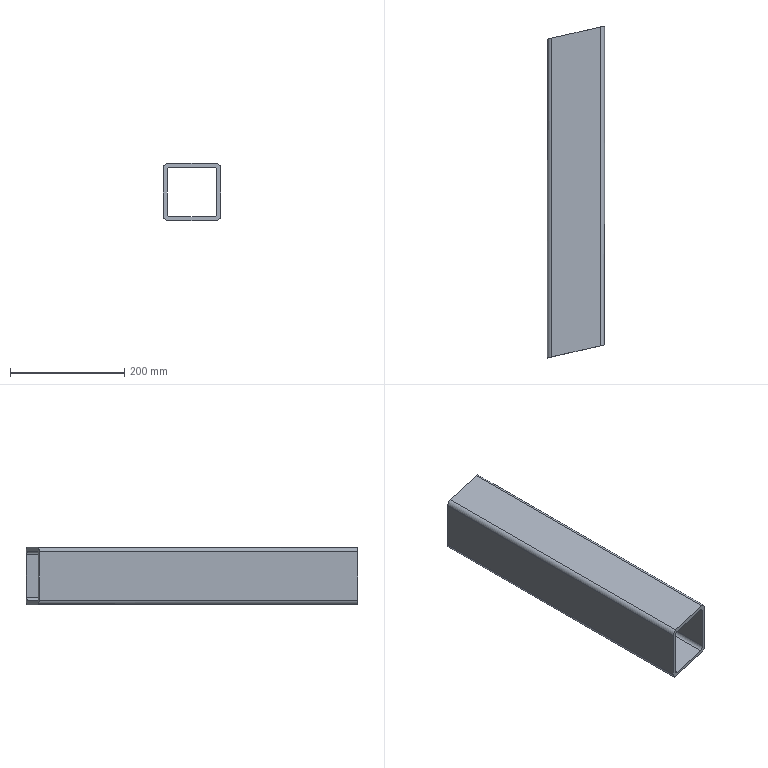Part | SolidWorks | features Extrusion 1, ICE 1 | 1 solid | 18 faces | box 100 x 582 x 100 mm | volume 1309220 mm3 | plane 10 | cylinder 8 | commonest cylinder face diameters 12.6 x4 15.75 x4
STEP:
#1=CARTESIAN_POINT('',(100.,291.,-90.6));
#2=VERTEX_POINT('',#1);
#3=CARTESIAN_POINT('',(100.,-268.,-90.6));
#4=VERTEX_POINT('',#3);
#5=CARTESIAN_POINT('',(100.,291.,-90.6));
#6=DIRECTION('',(0.,-1.,0.));
#7=VECTOR('',#6,1000.);
#8=LINE('',#5,#7);
#9=EDGE_CURVE('',#2,#4,#8,.T.);
#10=ORIENTED_EDGE('',*,*,#9,.T.);
#11=CARTESIAN_POINT('',(92.125,-269.811,-98.475));
#12=VERTEX_POINT('',#11);
#13=CARTESIAN_POINT('',(92.125,-269.811,-98.475));
#14=CARTESIAN_POINT('',(96.738,-268.75,-98.475));
#15=CARTESIAN_POINT('',(100.,-268.,-95.213));
#16=CARTESIAN_POINT('',(100.,-268.,-90.6));
#17=(BOUNDED_CURVE()B_SPLINE_CURVE(3,(#13,#14,#15,#16),.UNSPECIFIED.,.F.,.T.)B_SPLINE_CURVE_WITH_KNOTS((4,4),(1.571,3.142),.UNSPECIFIED.)CURVE()GEOMETRIC_REPRESENTATION_ITEM()RATIONAL_B_SPLINE_CURVE((1.,0.8047,0.8047,1.))REPRESENTATION_ITEM(''));
#18=EDGE_CURVE('',#12,#4,#17,.T.);
#19=ORIENTED_EDGE('',*,*,#18,.F.);
#20=CARTESIAN_POINT('',(92.125,289.189,-98.475));
#21=VERTEX_POINT('',#20);
#22=CARTESIAN_POINT('',(92.125,291.,-98.475));
#23=DIRECTION('',(0.,-1.,0.));
#24=VECTOR('',#23,1000.);
#25=LINE('',#22,#24);
#26=EDGE_CURVE('',#21,#12,#25,.T.);
#27=ORIENTED_EDGE('',*,*,#26,.F.);
#28=CARTESIAN_POINT('',(100.,291.,-90.6));
#29=CARTESIAN_POINT('',(100.,291.,-95.213));
#30=CARTESIAN_POINT('',(96.738,290.25,-98.475));
#31=CARTESIAN_POINT('',(92.125,289.189,-98.475));
#32=(BOUNDED_CURVE()B_SPLINE_CURVE(3,(#28,#29,#30,#31),.UNSPECIFIED.,.F.,.T.)B_SPLINE_CURVE_WITH_KNOTS((4,4),(3.142,4.712),.UNSPECIFIED.)CURVE()GEOMETRIC_REPRESENTATION_ITEM()RATIONAL_B_SPLINE_CURVE((1.,0.8047,0.8047,1.))REPRESENTATION_ITEM(''));
#33=EDGE_CURVE('',#2,#21,#32,.T.);
#34=ORIENTED_EDGE('',*,*,#33,.F.);
#35=EDGE_LOOP('',(#10,#19,#27,#34));
#36=FACE_OUTER_BOUND('',#35,.T.);
#37=CARTESIAN_POINT('',(92.125,291.,-90.6));
#38=DIRECTION('',(0.,-1.,0.));
#39=DIRECTION('',(0.,0.,-1.));
#40=AXIS2_PLACEMENT_3D('',#37,#38,#39);
#41=CYLINDRICAL_SURFACE('',#40,7.875);
#42=ADVANCED_FACE('',(#36),#41,.T.);
#43=ORIENTED_EDGE('',*,*,#26,.T.);
#44=CARTESIAN_POINT('',(7.875,-289.189,-98.475));
#45=VERTEX_POINT('',#44);
#46=CARTESIAN_POINT('',(0.,-291.,-98.475));
#47=DIRECTION('',(0.9746,0.2241,0.));
#48=VECTOR('',#47,1000.);
#49=LINE('',#46,#48);
#50=EDGE_CURVE('',#45,#12,#49,.T.);
#51=ORIENTED_EDGE('',*,*,#50,.F.);
#52=CARTESIAN_POINT('',(7.875,269.811,-98.475));
#53=VERTEX_POINT('',#52);
#54=CARTESIAN_POINT('',(7.875,291.,-98.475));
#55=DIRECTION('',(0.,-1.,0.));
#56=VECTOR('',#55,1000.);
#57=LINE('',#54,#56);
#58=EDGE_CURVE('',#53,#45,#57,.T.);
#59=ORIENTED_EDGE('',*,*,#58,.F.);
#60=CARTESIAN_POINT('',(100.,291.,-98.475));
#61=DIRECTION('',(-0.9746,-0.2241,0.));
#62=VECTOR('',#61,1000.);
#63=LINE('',#60,#62);
#64=EDGE_CURVE('',#21,#53,#63,.T.);
#65=ORIENTED_EDGE('',*,*,#64,.F.);
#66=EDGE_LOOP('',(#43,#51,#59,#65));
#67=FACE_OUTER_BOUND('',#66,.T.);
#68=CARTESIAN_POINT('',(92.125,291.,-98.475));
#69=DIRECTION('',(0.,0.,1.));
#70=DIRECTION('',(1.,0.,0.));
#71=AXIS2_PLACEMENT_3D('',#68,#69,#70);
#72=PLANE('',#71);
#73=ADVANCED_FACE('',(#67),#72,.F.);
#74=ORIENTED_EDGE('',*,*,#58,.T.);
#75=CARTESIAN_POINT('',(0.,-291.,-90.6));
#76=VERTEX_POINT('',#75);
#77=CARTESIAN_POINT('',(0.,-291.,-90.6));
#78=CARTESIAN_POINT('',(0.,-291.,-95.213));
#79=CARTESIAN_POINT('',(3.262,-290.25,-98.475));
#80=CARTESIAN_POINT('',(7.875,-289.189,-98.475));
#81=(BOUNDED_CURVE()B_SPLINE_CURVE(3,(#77,#78,#79,#80),.UNSPECIFIED.,.F.,.T.)B_SPLINE_CURVE_WITH_KNOTS((4,4),(0.,1.571),.UNSPECIFIED.)CURVE()GEOMETRIC_REPRESENTATION_ITEM()RATIONAL_B_SPLINE_CURVE((1.,0.8047,0.8047,1.))REPRESENTATION_ITEM(''));
#82=EDGE_CURVE('',#76,#45,#81,.T.);
#83=ORIENTED_EDGE('',*,*,#82,.F.);
#84=CARTESIAN_POINT('',(0.,268.,-90.6));
#85=VERTEX_POINT('',#84);
#86=CARTESIAN_POINT('',(0.,291.,-90.6));
#87=DIRECTION('',(0.,-1.,0.));
#88=VECTOR('',#87,1000.);
#89=LINE('',#86,#88);
#90=EDGE_CURVE('',#85,#76,#89,.T.);
#91=ORIENTED_EDGE('',*,*,#90,.F.);
#92=CARTESIAN_POINT('',(7.875,269.811,-98.475));
#93=CARTESIAN_POINT('',(3.262,268.75,-98.475));
#94=CARTESIAN_POINT('',(0.,268.,-95.213));
#95=CARTESIAN_POINT('',(0.,268.,-90.6));
#96=(BOUNDED_CURVE()B_SPLINE_CURVE(3,(#92,#93,#94,#95),.UNSPECIFIED.,.F.,.F.)B_SPLINE_CURVE_WITH_KNOTS((4,4),(4.712,6.283),.UNSPECIFIED.)CURVE()GEOMETRIC_REPRESENTATION_ITEM()RATIONAL_B_SPLINE_CURVE((1.,0.8047,0.8047,1.))REPRESENTATION_ITEM(''));
#97=EDGE_CURVE('',#53,#85,#96,.T.);
#98=ORIENTED_EDGE('',*,*,#97,.F.);
#99=EDGE_LOOP('',(#74,#83,#91,#98));
#100=FACE_OUTER_BOUND('',#99,.T.);
#101=CARTESIAN_POINT('',(7.875,291.,-90.6));
#102=DIRECTION('',(0.,-1.,0.));
#103=DIRECTION('',(0.,0.,-1.));
#104=AXIS2_PLACEMENT_3D('',#101,#102,#103);
#105=CYLINDRICAL_SURFACE('',#104,7.875);
#106=ADVANCED_FACE('',(#100),#105,.T.);
#107=CARTESIAN_POINT('',(0.,268.,-6.35));
#108=VERTEX_POINT('',#107);
#109=CARTESIAN_POINT('',(0.,-291.,-6.35));
#110=VERTEX_POINT('',#109);
#111=CARTESIAN_POINT('',(0.,291.,-6.35));
#112=DIRECTION('',(0.,-1.,0.));
#113=VECTOR('',#112,1000.);
#114=LINE('',#111,#113);
#115=EDGE_CURVE('',#108,#110,#114,.T.);
#116=ORIENTED_EDGE('',*,*,#115,.F.);
#117=CARTESIAN_POINT('',(0.,268.,-98.476));
#118=DIRECTION('',(0.,0.,1.));
#119=VECTOR('',#118,1000.);
#120=LINE('',#117,#119);
#121=EDGE_CURVE('',#85,#108,#120,.T.);
#122=ORIENTED_EDGE('',*,*,#121,.F.);
#123=ORIENTED_EDGE('',*,*,#90,.T.);
#124=CARTESIAN_POINT('',(0.,-291.,-6.35));
#125=DIRECTION('',(0.,0.,1.));
#126=VECTOR('',#125,1000.);
#127=LINE('',#124,#126);
#128=EDGE_CURVE('',#76,#110,#127,.T.);
#129=ORIENTED_EDGE('',*,*,#128,.T.);
#130=EDGE_LOOP('',(#116,#122,#123,#129));
#131=FACE_OUTER_BOUND('',#130,.T.);
#132=CARTESIAN_POINT('',(0.,291.,-6.35));
#133=DIRECTION('',(1.,0.,0.));
#134=DIRECTION('',(0.,0.,-1.));
#135=AXIS2_PLACEMENT_3D('',#132,#133,#134);
#136=PLANE('',#135);
#137=ADVANCED_FACE('',(#131),#136,.F.);
#138=ORIENTED_EDGE('',*,*,#115,.T.);
#139=CARTESIAN_POINT('',(7.875,-289.189,1.525));
#140=VERTEX_POINT('',#139);
#141=CARTESIAN_POINT('',(7.875,-289.189,1.525));
#142=CARTESIAN_POINT('',(3.262,-290.25,1.525));
#143=CARTESIAN_POINT('',(0.,-291.,-1.737));
#144=CARTESIAN_POINT('',(0.,-291.,-6.35));
#145=(BOUNDED_CURVE()B_SPLINE_CURVE(3,(#141,#142,#143,#144),.UNSPECIFIED.,.F.,.T.)B_SPLINE_CURVE_WITH_KNOTS((4,4),(4.712,6.283),.UNSPECIFIED.)CURVE()GEOMETRIC_REPRESENTATION_ITEM()RATIONAL_B_SPLINE_CURVE((1.,0.8047,0.8047,1.))REPRESENTATION_ITEM(''));
#146=EDGE_CURVE('',#140,#110,#145,.T.);
#147=ORIENTED_EDGE('',*,*,#146,.F.);
#148=CARTESIAN_POINT('',(7.875,269.811,1.525));
#149=VERTEX_POINT('',#148);
#150=CARTESIAN_POINT('',(7.875,291.,1.525));
#151=DIRECTION('',(0.,-1.,0.));
#152=VECTOR('',#151,1000.);
#153=LINE('',#150,#152);
#154=EDGE_CURVE('',#149,#140,#153,.T.);
#155=ORIENTED_EDGE('',*,*,#154,.F.);
#156=CARTESIAN_POINT('',(0.,268.,-6.35));
#157=CARTESIAN_POINT('',(0.,268.,-1.737));
#158=CARTESIAN_POINT('',(3.262,268.75,1.525));
#159=CARTESIAN_POINT('',(7.875,269.811,1.525));
#160=(BOUNDED_CURVE()B_SPLINE_CURVE(3,(#156,#157,#158,#159),.UNSPECIFIED.,.F.,.T.)B_SPLINE_CURVE_WITH_KNOTS((4,4),(0.,1.571),.UNSPECIFIED.)CURVE()GEOMETRIC_REPRESENTATION_ITEM()RATIONAL_B_SPLINE_CURVE((1.,0.8047,0.8047,1.))REPRESENTATION_ITEM(''));
#161=EDGE_CURVE('',#108,#149,#160,.T.);
#162=ORIENTED_EDGE('',*,*,#161,.F.);
#163=EDGE_LOOP('',(#138,#147,#155,#162));
#164=FACE_OUTER_BOUND('',#163,.T.);
#165=CARTESIAN_POINT('',(7.875,291.,-6.35));
#166=DIRECTION('',(0.,-1.,0.));
#167=DIRECTION('',(0.,0.,-1.));
#168=AXIS2_PLACEMENT_3D('',#165,#166,#167);
#169=CYLINDRICAL_SURFACE('',#168,7.875);
#170=ADVANCED_FACE('',(#164),#169,.T.);
#171=ORIENTED_EDGE('',*,*,#154,.T.);
#172=CARTESIAN_POINT('',(92.125,-269.811,1.525));
#173=VERTEX_POINT('',#172);
#174=CARTESIAN_POINT('',(0.,-291.,1.525));
#175=DIRECTION('',(-0.9746,-0.2241,0.));
#176=VECTOR('',#175,1000.);
#177=LINE('',#174,#176);
#178=EDGE_CURVE('',#173,#140,#177,.T.);
#179=ORIENTED_EDGE('',*,*,#178,.F.);
#180=CARTESIAN_POINT('',(92.125,289.189,1.525));
#181=VERTEX_POINT('',#180);
#182=CARTESIAN_POINT('',(92.125,291.,1.525));
#183=DIRECTION('',(0.,-1.,0.));
#184=VECTOR('',#183,1000.);
#185=LINE('',#182,#184);
#186=EDGE_CURVE('',#181,#173,#185,.T.);
#187=ORIENTED_EDGE('',*,*,#186,.F.);
#188=CARTESIAN_POINT('',(100.,291.,1.525));
#189=DIRECTION('',(0.9746,0.2241,0.));
#190=VECTOR('',#189,1000.);
#191=LINE('',#188,#190);
#192=EDGE_CURVE('',#149,#181,#191,.T.);
#193=ORIENTED_EDGE('',*,*,#192,.F.);
#194=EDGE_LOOP('',(#171,#179,#187,#193));
#195=FACE_OUTER_BOUND('',#194,.T.);
#196=CARTESIAN_POINT('',(7.875,291.,1.525));
#197=DIRECTION('',(0.,0.,-1.));
#198=DIRECTION('',(-1.,0.,0.));
#199=AXIS2_PLACEMENT_3D('',#196,#197,#198);
#200=PLANE('',#199);
#201=ADVANCED_FACE('',(#195),#200,.F.);
#202=ORIENTED_EDGE('',*,*,#186,.T.);
#203=CARTESIAN_POINT('',(100.,-268.,-6.35));
#204=VERTEX_POINT('',#203);
#205=CARTESIAN_POINT('',(100.,-268.,-6.35));
#206=CARTESIAN_POINT('',(100.,-268.,-1.737));
#207=CARTESIAN_POINT('',(96.738,-268.75,1.525));
#208=CARTESIAN_POINT('',(92.125,-269.811,1.525));
#209=(BOUNDED_CURVE()B_SPLINE_CURVE(3,(#205,#206,#207,#208),.UNSPECIFIED.,.F.,.T.)B_SPLINE_CURVE_WITH_KNOTS((4,4),(3.142,4.712),.UNSPECIFIED.)CURVE()GEOMETRIC_REPRESENTATION_ITEM()RATIONAL_B_SPLINE_CURVE((1.,0.8047,0.8047,1.))REPRESENTATION_ITEM(''));
#210=EDGE_CURVE('',#204,#173,#209,.T.);
#211=ORIENTED_EDGE('',*,*,#210,.F.);
#212=CARTESIAN_POINT('',(100.,291.,-6.35));
#213=VERTEX_POINT('',#212);
#214=CARTESIAN_POINT('',(100.,291.,-6.35));
#215=DIRECTION('',(0.,-1.,0.));
#216=VECTOR('',#215,1000.);
#217=LINE('',#214,#216);
#218=EDGE_CURVE('',#213,#204,#217,.T.);
#219=ORIENTED_EDGE('',*,*,#218,.F.);
#220=CARTESIAN_POINT('',(92.125,289.189,1.525));
#221=CARTESIAN_POINT('',(96.738,290.25,1.525));
#222=CARTESIAN_POINT('',(100.,291.,-1.737));
#223=CARTESIAN_POINT('',(100.,291.,-6.35));
#224=(BOUNDED_CURVE()B_SPLINE_CURVE(3,(#220,#221,#222,#223),.UNSPECIFIED.,.F.,.T.)B_SPLINE_CURVE_WITH_KNOTS((4,4),(1.571,3.142),.UNSPECIFIED.)CURVE()GEOMETRIC_REPRESENTATION_ITEM()RATIONAL_B_SPLINE_CURVE((1.,0.8047,0.8047,1.))REPRESENTATION_ITEM(''));
#225=EDGE_CURVE('',#181,#213,#224,.T.);
#226=ORIENTED_EDGE('',*,*,#225,.F.);
#227=EDGE_LOOP('',(#202,#211,#219,#226));
#228=FACE_OUTER_BOUND('',#227,.T.);
#229=CARTESIAN_POINT('',(92.125,291.,-6.35));
#230=DIRECTION('',(0.,-1.,0.));
#231=DIRECTION('',(0.,0.,-1.));
#232=AXIS2_PLACEMENT_3D('',#229,#230,#231);
#233=CYLINDRICAL_SURFACE('',#232,7.875);
#234=ADVANCED_FACE('',(#228),#233,.T.);
#235=ORIENTED_EDGE('',*,*,#218,.T.);
#236=CARTESIAN_POINT('',(100.,-268.,-98.476));
#237=DIRECTION('',(0.,0.,1.));
#238=VECTOR('',#237,1000.);
#239=LINE('',#236,#238);
#240=EDGE_CURVE('',#4,#204,#239,.T.);
#241=ORIENTED_EDGE('',*,*,#240,.F.);
#242=ORIENTED_EDGE('',*,*,#9,.F.);
#243=CARTESIAN_POINT('',(100.,291.,-90.6));
#244=DIRECTION('',(0.,0.,-1.));
#245=VECTOR('',#244,1000.);
#246=LINE('',#243,#245);
#247=EDGE_CURVE('',#213,#2,#246,.T.);
#248=ORIENTED_EDGE('',*,*,#247,.F.);
#249=EDGE_LOOP('',(#235,#241,#242,#248));
#250=FACE_OUTER_BOUND('',#249,.T.);
#251=CARTESIAN_POINT('',(100.,291.,-90.6));
#252=DIRECTION('',(-1.,0.,0.));
#253=DIRECTION('',(0.,0.,1.));
#254=AXIS2_PLACEMENT_3D('',#251,#252,#253);
#255=PLANE('',#254);
#256=ADVANCED_FACE('',(#250),#255,.F.);
#257=CARTESIAN_POINT('',(6.3,-289.551,-85.875));
#258=VERTEX_POINT('',#257);
#259=CARTESIAN_POINT('',(12.6,-288.102,-92.175));
#260=VERTEX_POINT('',#259);
#261=CARTESIAN_POINT('',(6.3,-289.551,-85.875));
#262=CARTESIAN_POINT('',(6.3,-289.551,-89.565));
#263=CARTESIAN_POINT('',(8.91,-288.951,-92.175));
#264=CARTESIAN_POINT('',(12.6,-288.102,-92.175));
#265=(BOUNDED_CURVE()B_SPLINE_CURVE(3,(#261,#262,#263,#264),.UNSPECIFIED.,.F.,.T.)B_SPLINE_CURVE_WITH_KNOTS((4,4),(0.,1.571),.UNSPECIFIED.)CURVE()GEOMETRIC_REPRESENTATION_ITEM()RATIONAL_B_SPLINE_CURVE((1.,0.8047,0.8047,1.))REPRESENTATION_ITEM(''));
#266=EDGE_CURVE('',#258,#260,#265,.T.);
#267=ORIENTED_EDGE('',*,*,#266,.T.);
#268=CARTESIAN_POINT('',(12.6,270.898,-92.175));
#269=VERTEX_POINT('',#268);
#270=CARTESIAN_POINT('',(12.6,291.,-92.175));
#271=DIRECTION('',(0.,-1.,0.));
#272=VECTOR('',#271,1000.);
#273=LINE('',#270,#272);
#274=EDGE_CURVE('',#269,#260,#273,.T.);
#275=ORIENTED_EDGE('',*,*,#274,.F.);
#276=CARTESIAN_POINT('',(6.3,269.449,-85.875));
#277=VERTEX_POINT('',#276);
#278=CARTESIAN_POINT('',(12.6,270.898,-92.175));
#279=CARTESIAN_POINT('',(8.91,270.049,-92.175));
#280=CARTESIAN_POINT('',(6.3,269.449,-89.565));
#281=CARTESIAN_POINT('',(6.3,269.449,-85.875));
#282=(BOUNDED_CURVE()B_SPLINE_CURVE(3,(#278,#279,#280,#281),.UNSPECIFIED.,.F.,.T.)B_SPLINE_CURVE_WITH_KNOTS((4,4),(4.712,6.283),.UNSPECIFIED.)CURVE()GEOMETRIC_REPRESENTATION_ITEM()RATIONAL_B_SPLINE_CURVE((1.,0.8047,0.8047,1.))REPRESENTATION_ITEM(''));
#283=EDGE_CURVE('',#269,#277,#282,.T.);
#284=ORIENTED_EDGE('',*,*,#283,.T.);
#285=CARTESIAN_POINT('',(6.3,291.,-85.875));
#286=DIRECTION('',(0.,-1.,0.));
#287=VECTOR('',#286,1000.);
#288=LINE('',#285,#287);
#289=EDGE_CURVE('',#277,#258,#288,.T.);
#290=ORIENTED_EDGE('',*,*,#289,.T.);
#291=EDGE_LOOP('',(#267,#275,#284,#290));
#292=FACE_OUTER_BOUND('',#291,.T.);
#293=CARTESIAN_POINT('',(12.6,291.,-85.875));
#294=DIRECTION('',(0.,-1.,0.));
#295=DIRECTION('',(0.,0.,-1.));
#296=AXIS2_PLACEMENT_3D('',#293,#294,#295);
#297=CYLINDRICAL_SURFACE('',#296,6.3);
#298=ADVANCED_FACE('',(#292),#297,.F.);
#299=CARTESIAN_POINT('',(6.3,-289.551,-11.075));
#300=VERTEX_POINT('',#299);
#301=CARTESIAN_POINT('',(6.3,-289.551,-98.476));
#302=DIRECTION('',(0.,0.,-1.));
#303=VECTOR('',#302,1000.);
#304=LINE('',#301,#303);
#305=EDGE_CURVE('',#300,#258,#304,.T.);
#306=ORIENTED_EDGE('',*,*,#305,.T.);
#307=ORIENTED_EDGE('',*,*,#289,.F.);
#308=CARTESIAN_POINT('',(6.3,269.449,-11.075));
#309=VERTEX_POINT('',#308);
#310=CARTESIAN_POINT('',(6.3,269.449,-98.476));
#311=DIRECTION('',(0.,0.,1.));
#312=VECTOR('',#311,1000.);
#313=LINE('',#310,#312);
#314=EDGE_CURVE('',#277,#309,#313,.T.);
#315=ORIENTED_EDGE('',*,*,#314,.T.);
#316=CARTESIAN_POINT('',(6.3,291.,-11.075));
#317=DIRECTION('',(0.,-1.,0.));
#318=VECTOR('',#317,1000.);
#319=LINE('',#316,#318);
#320=EDGE_CURVE('',#309,#300,#319,.T.);
#321=ORIENTED_EDGE('',*,*,#320,.T.);
#322=EDGE_LOOP('',(#306,#307,#315,#321));
#323=FACE_OUTER_BOUND('',#322,.T.);
#324=CARTESIAN_POINT('',(6.3,291.,-11.075));
#325=DIRECTION('',(1.,0.,0.));
#326=DIRECTION('',(0.,0.,-1.));
#327=AXIS2_PLACEMENT_3D('',#324,#325,#326);
#328=PLANE('',#327);
#329=ADVANCED_FACE('',(#323),#328,.T.);
#330=CARTESIAN_POINT('',(12.6,-288.102,-4.775));
#331=VERTEX_POINT('',#330);
#332=CARTESIAN_POINT('',(12.6,-288.102,-4.775));
#333=CARTESIAN_POINT('',(8.91,-288.951,-4.775));
#334=CARTESIAN_POINT('',(6.3,-289.551,-7.385));
#335=CARTESIAN_POINT('',(6.3,-289.551,-11.075));
#336=(BOUNDED_CURVE()B_SPLINE_CURVE(3,(#332,#333,#334,#335),.UNSPECIFIED.,.F.,.T.)B_SPLINE_CURVE_WITH_KNOTS((4,4),(4.712,6.283),.UNSPECIFIED.)CURVE()GEOMETRIC_REPRESENTATION_ITEM()RATIONAL_B_SPLINE_CURVE((1.,0.8047,0.8047,1.))REPRESENTATION_ITEM(''));
#337=EDGE_CURVE('',#331,#300,#336,.T.);
#338=ORIENTED_EDGE('',*,*,#337,.T.);
#339=ORIENTED_EDGE('',*,*,#320,.F.);
#340=CARTESIAN_POINT('',(12.6,270.898,-4.775));
#341=VERTEX_POINT('',#340);
#342=CARTESIAN_POINT('',(6.3,269.449,-11.075));
#343=CARTESIAN_POINT('',(6.3,269.449,-7.385));
#344=CARTESIAN_POINT('',(8.91,270.049,-4.775));
#345=CARTESIAN_POINT('',(12.6,270.898,-4.775));
#346=(BOUNDED_CURVE()B_SPLINE_CURVE(3,(#342,#343,#344,#345),.UNSPECIFIED.,.F.,.T.)B_SPLINE_CURVE_WITH_KNOTS((4,4),(0.,1.571),.UNSPECIFIED.)CURVE()GEOMETRIC_REPRESENTATION_ITEM()RATIONAL_B_SPLINE_CURVE((1.,0.8047,0.8047,1.))REPRESENTATION_ITEM(''));
#347=EDGE_CURVE('',#309,#341,#346,.T.);
#348=ORIENTED_EDGE('',*,*,#347,.T.);
#349=CARTESIAN_POINT('',(12.6,291.,-4.775));
#350=DIRECTION('',(0.,-1.,0.));
#351=VECTOR('',#350,1000.);
#352=LINE('',#349,#351);
#353=EDGE_CURVE('',#341,#331,#352,.T.);
#354=ORIENTED_EDGE('',*,*,#353,.T.);
#355=EDGE_LOOP('',(#338,#339,#348,#354));
#356=FACE_OUTER_BOUND('',#355,.T.);
#357=CARTESIAN_POINT('',(12.6,291.,-11.075));
#358=DIRECTION('',(0.,-1.,0.));
#359=DIRECTION('',(0.,0.,-1.));
#360=AXIS2_PLACEMENT_3D('',#357,#358,#359);
#361=CYLINDRICAL_SURFACE('',#360,6.3);
#362=ADVANCED_FACE('',(#356),#361,.F.);
#363=CARTESIAN_POINT('',(87.4,-270.898,-4.775));
#364=VERTEX_POINT('',#363);
#365=CARTESIAN_POINT('',(0.,-291.,-4.775));
#366=DIRECTION('',(-0.9746,-0.2241,0.));
#367=VECTOR('',#366,1000.);
#368=LINE('',#365,#367);
#369=EDGE_CURVE('',#364,#331,#368,.T.);
#370=ORIENTED_EDGE('',*,*,#369,.T.);
#371=ORIENTED_EDGE('',*,*,#353,.F.);
#372=CARTESIAN_POINT('',(87.4,288.102,-4.775));
#373=VERTEX_POINT('',#372);
#374=CARTESIAN_POINT('',(100.,291.,-4.775));
#375=DIRECTION('',(0.9746,0.2241,0.));
#376=VECTOR('',#375,1000.);
#377=LINE('',#374,#376);
#378=EDGE_CURVE('',#341,#373,#377,.T.);
#379=ORIENTED_EDGE('',*,*,#378,.T.);
#380=CARTESIAN_POINT('',(87.4,291.,-4.775));
#381=DIRECTION('',(0.,-1.,0.));
#382=VECTOR('',#381,1000.);
#383=LINE('',#380,#382);
#384=EDGE_CURVE('',#373,#364,#383,.T.);
#385=ORIENTED_EDGE('',*,*,#384,.T.);
#386=EDGE_LOOP('',(#370,#371,#379,#385));
#387=FACE_OUTER_BOUND('',#386,.T.);
#388=CARTESIAN_POINT('',(12.6,291.,-4.775));
#389=DIRECTION('',(0.,0.,-1.));
#390=DIRECTION('',(-1.,0.,0.));
#391=AXIS2_PLACEMENT_3D('',#388,#389,#390);
#392=PLANE('',#391);
#393=ADVANCED_FACE('',(#387),#392,.T.);
#394=CARTESIAN_POINT('',(93.7,-269.449,-11.075));
#395=VERTEX_POINT('',#394);
#396=CARTESIAN_POINT('',(93.7,-269.449,-11.075));
#397=CARTESIAN_POINT('',(93.7,-269.449,-7.385));
#398=CARTESIAN_POINT('',(91.09,-270.049,-4.775));
#399=CARTESIAN_POINT('',(87.4,-270.898,-4.775));
#400=(BOUNDED_CURVE()B_SPLINE_CURVE(3,(#396,#397,#398,#399),.UNSPECIFIED.,.F.,.F.)B_SPLINE_CURVE_WITH_KNOTS((4,4),(3.142,4.712),.UNSPECIFIED.)CURVE()GEOMETRIC_REPRESENTATION_ITEM()RATIONAL_B_SPLINE_CURVE((1.,0.8047,0.8047,1.))REPRESENTATION_ITEM(''));
#401=EDGE_CURVE('',#395,#364,#400,.T.);
#402=ORIENTED_EDGE('',*,*,#401,.T.);
#403=ORIENTED_EDGE('',*,*,#384,.F.);
#404=CARTESIAN_POINT('',(93.7,289.551,-11.075));
#405=VERTEX_POINT('',#404);
#406=CARTESIAN_POINT('',(87.4,288.102,-4.775));
#407=CARTESIAN_POINT('',(91.09,288.951,-4.775));
#408=CARTESIAN_POINT('',(93.7,289.551,-7.385));
#409=CARTESIAN_POINT('',(93.7,289.551,-11.075));
#410=(BOUNDED_CURVE()B_SPLINE_CURVE(3,(#406,#407,#408,#409),.UNSPECIFIED.,.F.,.T.)B_SPLINE_CURVE_WITH_KNOTS((4,4),(1.571,3.142),.UNSPECIFIED.)CURVE()GEOMETRIC_REPRESENTATION_ITEM()RATIONAL_B_SPLINE_CURVE((1.,0.8047,0.8047,1.))REPRESENTATION_ITEM(''));
#411=EDGE_CURVE('',#373,#405,#410,.T.);
#412=ORIENTED_EDGE('',*,*,#411,.T.);
#413=CARTESIAN_POINT('',(93.7,291.,-11.075));
#414=DIRECTION('',(0.,-1.,0.));
#415=VECTOR('',#414,1000.);
#416=LINE('',#413,#415);
#417=EDGE_CURVE('',#405,#395,#416,.T.);
#418=ORIENTED_EDGE('',*,*,#417,.T.);
#419=EDGE_LOOP('',(#402,#403,#412,#418));
#420=FACE_OUTER_BOUND('',#419,.T.);
#421=CARTESIAN_POINT('',(87.4,291.,-11.075));
#422=DIRECTION('',(0.,-1.,0.));
#423=DIRECTION('',(0.,0.,-1.));
#424=AXIS2_PLACEMENT_3D('',#421,#422,#423);
#425=CYLINDRICAL_SURFACE('',#424,6.3);
#426=ADVANCED_FACE('',(#420),#425,.F.);
#427=CARTESIAN_POINT('',(93.7,-269.449,-85.875));
#428=VERTEX_POINT('',#427);
#429=CARTESIAN_POINT('',(93.7,-269.449,-98.476));
#430=DIRECTION('',(0.,0.,1.));
#431=VECTOR('',#430,1000.);
#432=LINE('',#429,#431);
#433=EDGE_CURVE('',#428,#395,#432,.T.);
#434=ORIENTED_EDGE('',*,*,#433,.T.);
#435=ORIENTED_EDGE('',*,*,#417,.F.);
#436=CARTESIAN_POINT('',(93.7,289.551,-85.875));
#437=VERTEX_POINT('',#436);
#438=CARTESIAN_POINT('',(93.7,289.551,-98.476));
#439=DIRECTION('',(0.,0.,-1.));
#440=VECTOR('',#439,1000.);
#441=LINE('',#438,#440);
#442=EDGE_CURVE('',#405,#437,#441,.T.);
#443=ORIENTED_EDGE('',*,*,#442,.T.);
#444=CARTESIAN_POINT('',(93.7,291.,-85.875));
#445=DIRECTION('',(0.,-1.,0.));
#446=VECTOR('',#445,1000.);
#447=LINE('',#444,#446);
#448=EDGE_CURVE('',#437,#428,#447,.T.);
#449=ORIENTED_EDGE('',*,*,#448,.T.);
#450=EDGE_LOOP('',(#434,#435,#443,#449));
#451=FACE_OUTER_BOUND('',#450,.T.);
#452=CARTESIAN_POINT('',(93.7,291.,-85.875));
#453=DIRECTION('',(-1.,0.,0.));
#454=DIRECTION('',(0.,0.,1.));
#455=AXIS2_PLACEMENT_3D('',#452,#453,#454);
#456=PLANE('',#455);
#457=ADVANCED_FACE('',(#451),#456,.T.);
#458=CARTESIAN_POINT('',(87.4,-270.898,-92.175));
#459=VERTEX_POINT('',#458);
#460=CARTESIAN_POINT('',(87.4,-270.898,-92.175));
#461=CARTESIAN_POINT('',(91.09,-270.049,-92.175));
#462=CARTESIAN_POINT('',(93.7,-269.449,-89.565));
#463=CARTESIAN_POINT('',(93.7,-269.449,-85.875));
#464=(BOUNDED_CURVE()B_SPLINE_CURVE(3,(#460,#461,#462,#463),.UNSPECIFIED.,.F.,.T.)B_SPLINE_CURVE_WITH_KNOTS((4,4),(1.571,3.142),.UNSPECIFIED.)CURVE()GEOMETRIC_REPRESENTATION_ITEM()RATIONAL_B_SPLINE_CURVE((1.,0.8047,0.8047,1.))REPRESENTATION_ITEM(''));
#465=EDGE_CURVE('',#459,#428,#464,.T.);
#466=ORIENTED_EDGE('',*,*,#465,.T.);
#467=ORIENTED_EDGE('',*,*,#448,.F.);
#468=CARTESIAN_POINT('',(87.4,288.102,-92.175));
#469=VERTEX_POINT('',#468);
#470=CARTESIAN_POINT('',(93.7,289.551,-85.875));
#471=CARTESIAN_POINT('',(93.7,289.551,-89.565));
#472=CARTESIAN_POINT('',(91.09,288.951,-92.175));
#473=CARTESIAN_POINT('',(87.4,288.102,-92.175));
#474=(BOUNDED_CURVE()B_SPLINE_CURVE(3,(#470,#471,#472,#473),.UNSPECIFIED.,.F.,.T.)B_SPLINE_CURVE_WITH_KNOTS((4,4),(3.142,4.712),.UNSPECIFIED.)CURVE()GEOMETRIC_REPRESENTATION_ITEM()RATIONAL_B_SPLINE_CURVE((1.,0.8047,0.8047,1.))REPRESENTATION_ITEM(''));
#475=EDGE_CURVE('',#437,#469,#474,.T.);
#476=ORIENTED_EDGE('',*,*,#475,.T.);
#477=CARTESIAN_POINT('',(87.4,291.,-92.175));
#478=DIRECTION('',(0.,-1.,0.));
#479=VECTOR('',#478,1000.);
#480=LINE('',#477,#479);
#481=EDGE_CURVE('',#469,#459,#480,.T.);
#482=ORIENTED_EDGE('',*,*,#481,.T.);
#483=EDGE_LOOP('',(#466,#467,#476,#482));
#484=FACE_OUTER_BOUND('',#483,.T.);
#485=CARTESIAN_POINT('',(87.4,291.,-85.875));
#486=DIRECTION('',(0.,-1.,0.));
#487=DIRECTION('',(0.,0.,-1.));
#488=AXIS2_PLACEMENT_3D('',#485,#486,#487);
#489=CYLINDRICAL_SURFACE('',#488,6.3);
#490=ADVANCED_FACE('',(#484),#489,.F.);
#491=CARTESIAN_POINT('',(0.,-291.,-92.175));
#492=DIRECTION('',(0.9746,0.2241,0.));
#493=VECTOR('',#492,1000.);
#494=LINE('',#491,#493);
#495=EDGE_CURVE('',#260,#459,#494,.T.);
#496=ORIENTED_EDGE('',*,*,#495,.T.);
#497=ORIENTED_EDGE('',*,*,#481,.F.);
#498=CARTESIAN_POINT('',(100.,291.,-92.175));
#499=DIRECTION('',(-0.9746,-0.2241,0.));
#500=VECTOR('',#499,1000.);
#501=LINE('',#498,#500);
#502=EDGE_CURVE('',#469,#269,#501,.T.);
#503=ORIENTED_EDGE('',*,*,#502,.T.);
#504=ORIENTED_EDGE('',*,*,#274,.T.);
#505=EDGE_LOOP('',(#496,#497,#503,#504));
#506=FACE_OUTER_BOUND('',#505,.T.);
#507=CARTESIAN_POINT('',(87.4,291.,-92.175));
#508=DIRECTION('',(0.,0.,1.));
#509=DIRECTION('',(1.,0.,0.));
#510=AXIS2_PLACEMENT_3D('',#507,#508,#509);
#511=PLANE('',#510);
#512=ADVANCED_FACE('',(#506),#511,.T.);
#513=ORIENTED_EDGE('',*,*,#502,.F.);
#514=ORIENTED_EDGE('',*,*,#475,.F.);
#515=ORIENTED_EDGE('',*,*,#442,.F.);
#516=ORIENTED_EDGE('',*,*,#411,.F.);
#517=ORIENTED_EDGE('',*,*,#378,.F.);
#518=ORIENTED_EDGE('',*,*,#347,.F.);
#519=ORIENTED_EDGE('',*,*,#314,.F.);
#520=ORIENTED_EDGE('',*,*,#283,.F.);
#521=EDGE_LOOP('',(#513,#514,#515,#516,#517,#518,#519,#520));
#522=FACE_BOUND('',#521,.T.);
#523=ORIENTED_EDGE('',*,*,#33,.T.);
#524=ORIENTED_EDGE('',*,*,#64,.T.);
#525=ORIENTED_EDGE('',*,*,#97,.T.);
#526=ORIENTED_EDGE('',*,*,#121,.T.);
#527=ORIENTED_EDGE('',*,*,#161,.T.);
#528=ORIENTED_EDGE('',*,*,#192,.T.);
#529=ORIENTED_EDGE('',*,*,#225,.T.);
#530=ORIENTED_EDGE('',*,*,#247,.T.);
#531=EDGE_LOOP('',(#523,#524,#525,#526,#527,#528,#529,#530));
#532=FACE_OUTER_BOUND('',#531,.T.);
#533=CARTESIAN_POINT('',(100.,291.,-98.476));
#534=DIRECTION('',(0.2241,-0.9746,0.));
#535=DIRECTION('',(0.9746,0.2241,0.));
#536=AXIS2_PLACEMENT_3D('',#533,#534,#535);
#537=PLANE('',#536);
#538=ADVANCED_FACE('',(#522,#532),#537,.F.);
#539=ORIENTED_EDGE('',*,*,#305,.F.);
#540=ORIENTED_EDGE('',*,*,#337,.F.);
#541=ORIENTED_EDGE('',*,*,#369,.F.);
#542=ORIENTED_EDGE('',*,*,#401,.F.);
#543=ORIENTED_EDGE('',*,*,#433,.F.);
#544=ORIENTED_EDGE('',*,*,#465,.F.);
#545=ORIENTED_EDGE('',*,*,#495,.F.);
#546=ORIENTED_EDGE('',*,*,#266,.F.);
#547=EDGE_LOOP('',(#539,#540,#541,#542,#543,#544,#545,#546));
#548=FACE_BOUND('',#547,.T.);
#549=ORIENTED_EDGE('',*,*,#18,.T.);
#550=ORIENTED_EDGE('',*,*,#240,.T.);
#551=ORIENTED_EDGE('',*,*,#210,.T.);
#552=ORIENTED_EDGE('',*,*,#178,.T.);
#553=ORIENTED_EDGE('',*,*,#146,.T.);
#554=ORIENTED_EDGE('',*,*,#128,.F.);
#555=ORIENTED_EDGE('',*,*,#82,.T.);
#556=ORIENTED_EDGE('',*,*,#50,.T.);
#557=EDGE_LOOP('',(#549,#550,#551,#552,#553,#554,#555,#556));
#558=FACE_OUTER_BOUND('',#557,.T.);
#559=CARTESIAN_POINT('',(0.,-291.,-98.476));
#560=DIRECTION('',(-0.2241,0.9746,0.));
#561=DIRECTION('',(-0.9746,-0.2241,0.));
#562=AXIS2_PLACEMENT_3D('',#559,#560,#561);
#563=PLANE('',#562);
#564=ADVANCED_FACE('',(#548,#558),#563,.F.);
#565=CLOSED_SHELL('',(#42,#73,#106,#137,#170,#201,#234,#256,#298,#329,#362,#393,#426,#457,#490,#512,#538,#564));
#566=MANIFOLD_SOLID_BREP('',#565);
#567=CARTESIAN_POINT('',(0.,0.,0.));
#568=DIRECTION('',(0.,0.,1.));
#569=DIRECTION('',(1.,0.,0.));
#570=AXIS2_PLACEMENT_3D('',#567,#568,#569);
#571=(LENGTH_UNIT()NAMED_UNIT(*)SI_UNIT(.MILLI.,.METRE.));
#572=UNCERTAINTY_MEASURE_WITH_UNIT(LENGTH_MEASURE(0.00001),#571,'','');
#573=(NAMED_UNIT(*)PLANE_ANGLE_UNIT()SI_UNIT($,.RADIAN.));
#574=(NAMED_UNIT(*)SI_UNIT($,.STERADIAN.)SOLID_ANGLE_UNIT());
#575=(GEOMETRIC_REPRESENTATION_CONTEXT(3)GLOBAL_UNCERTAINTY_ASSIGNED_CONTEXT((#572))GLOBAL_UNIT_ASSIGNED_CONTEXT((#571,#573,#574))REPRESENTATION_CONTEXT('',''));
#576=ADVANCED_BREP_SHAPE_REPRESENTATION('',(#566,#570),#575);